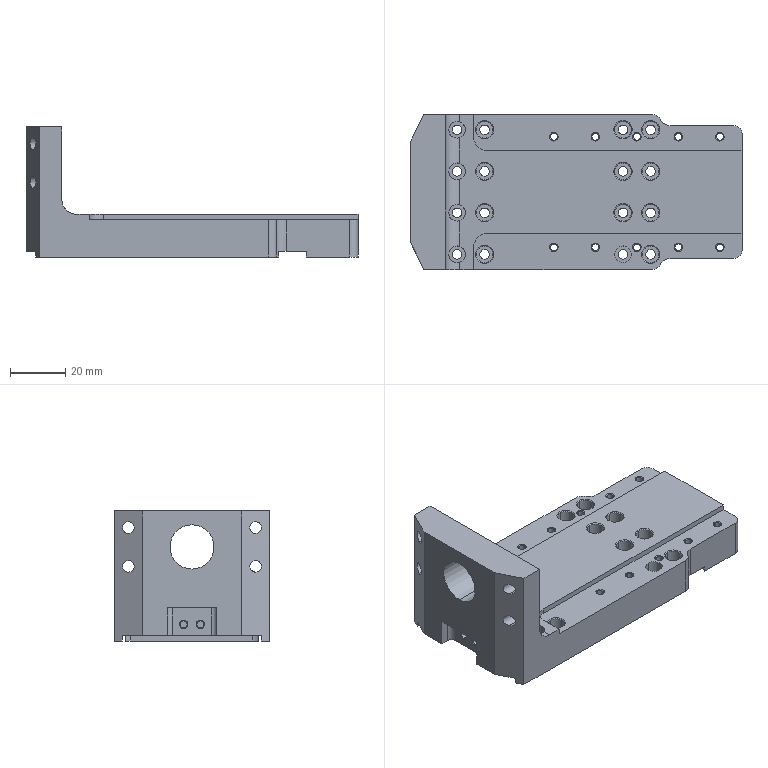CAM job | NX | 3-axis milling, drilling | part box 120 x 56 x 47 mm | stock box 126 x 62 x 48 mm
Tools:
number,name,description,diameter,corner_radius,flute_length,length,flutes
1,D63,Milling Tool-5 Parameters,63.0,0.0,50.0,75.0,2
10,D10,Milling Tool-5 Parameters,10.0,0.0,50.0,75.0,2
7,D6A45,Milling Tool-5 Parameters,6.0,0.0,3.0,3.0,2
15,3.5ZT,Drilling Tool,3.5,0.0,35.0,50.0,2
12,2.5ZT,Drilling Tool,2.5,0.0,35.0,50.0,2
13,M3,Milling Tool-5 Parameters,2.5,0.0,30.0,30.0,4
11,D10JING,Milling Tool-5 Parameters,10.0,0.0,50.0,75.0,2
5,D6R0.5,Milling Tool-5 Parameters,6.0,0.5,50.0,75.0,2
4,D4,Milling Tool-5 Parameters,4.0,0.0,50.0,75.0,2
Operations:
program,operation,operation_type,tool,method,geometry_group,spindle_rpm,surface_speed,feed_per_tooth,feed_cut,feed_plunge,cut_length_mm,path_length_mm,cut_time_min,machine_time_min
1-60-50-125毛胚,FLOOR_WALL,VolumeBased25DMillingOperation,D63,METHOD,A,6500.0,1286.0,0.0962,1250.0,100.0,201.0,255.0,0.1608,0.1662
1-60-50-125毛胚,ADAPTIVE_MILLING,CavityMilling,D10,METHOD,A,7000.0,219.0,0.2143,3000.0,1000.0,34056.001,39676.6,11.428,11.99
1-60-50-125毛胚,DRILLING_COPY_1,Operation,D6A45,METHOD,A,3000.0,56.0,0.0333,200.0,0.0,118.3,770.717,0.5915,0.6567
1-60-50-125毛胚,DRILLING_COPY_1_COPY_COPY_2,Operation,3.5ZT,METHOD,A,2000.0,15.0,0.0375,150.0,0.0,288.824,971.043,1.925,1.994
1-60-50-125毛胚,DRILLING_COPY_1_COPY,Operation,2.5ZT,METHOD,A,2000.0,15.0,0.0375,150.0,0.0,171.511,659.51,1.143,1.192
1-60-50-125毛胚,DRILLING_COPY_1_COPY_COPY,Operation,M3,METHOD,A,200.0,1.0,0.125,100.0,0.0,154.0,624.489,1.54,1.587
1-60-50-125毛胚,ZLEVEL_PROFILE_COPY_COPY_1_COPY_COPY_COPY_1,ZLevelMilling,D10JING,METHOD,A,7000.0,219.0,0.0714,1000.0,100.0,329.818,443.008,0.3298,0.3411
1-60-50-125毛胚,ZLEVEL_PROFILE_COPY_COPY_1_COPY_COPY_COPY_1_COPY,ZLevelMilling,D10JING,METHOD,A,7000.0,219.0,0.0714,1000.0,100.0,371.269,525.269,0.3713,0.3867
1-60-50-125毛胚,FLOOR_WALL_1_COPY_1,VolumeBased25DMillingOperation,D10JING,METHOD,A,7000.0,87.0,0.0714,1000.0,100.0,2056.585,2578.188,2.057,2.11
1-60-50-125毛胚,ZLEVEL_PROFILE_COPY_COPY_1_COPY_COPY_2_COPY_1,ZLevelMilling,D6R0.5,METHOD,A,7000.0,131.0,0.2143,3000.0,100.0,5317.882,5435.982,1.773,1.784
1-60-50-125毛胚,HOLE_MILLING,CylinderMilling,D4,METHOD,A,7000.0,131.0,0.1071,1500.0,100.0,3084.694,5407.725,2.057,2.289
1-60-50-125毛胚,ZLEVEL_PROFILE_COPY_1_COPY_COPY_COPY_COPY_2_COPY,ZLevelMilling,D6A45,METHOD,A,7000.0,131.0,0.0714,1000.0,1000.0,139.461,201.461,0.1395,0.1457
1-60-50-125毛胚,ZLEVEL_PROFILE_COPY_1_COPY_COPY_COPY_COPY_2_COPY_COPY,ZLevelMilling,D6A45,METHOD,A,7000.0,131.0,0.0714,1000.0,1000.0,396.038,2162.179,0.396,0.5727
1-60-50-125毛胚,ZLEVEL_PROFILE_COPY_1_COPY_COPY_COPY_COPY_2_COPY_COPY_COPY,ZLevelMilling,D6A45,METHOD,A,7000.0,131.0,0.0714,1000.0,1000.0,356.36,3280.907,0.3564,0.6488